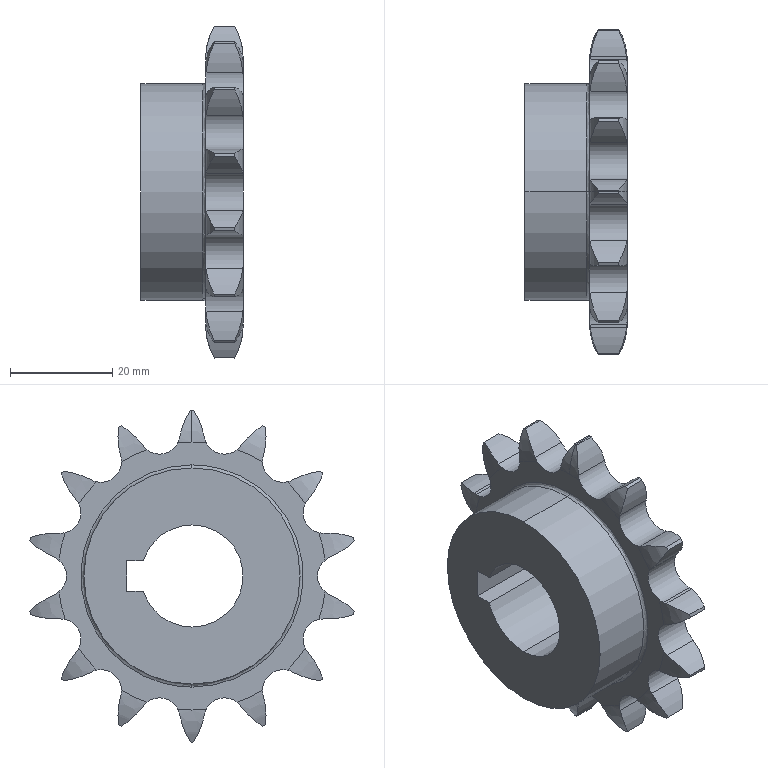Part | STEP file | short pitch roller chain wheel_s_iso_Chain wheel ISO - 14Z 08A-1 --14SB75H20L20.0S1 | 1 solid | 108 faces | box 20.001 x 63.542 x 65.028 mm | volume 28318 mm3 | cylinder 70 | spline 32 | plane 6 | commonest cylinder face diameters 30.413 x30 7.999 x20 65.028 x15 20 x3 42.33 x2